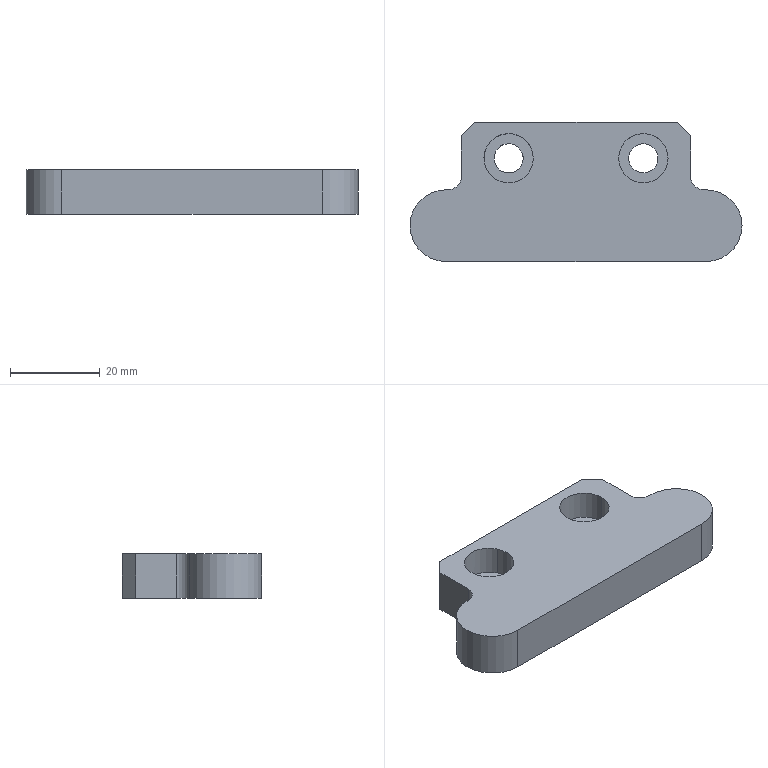Part | STEP file | 1_id1094_x_t | 1 solid | 28 faces | box 73.936 x 31 x 10 mm | volume 16212 mm3 | cylinder 16 | plane 12 | commonest cylinder face diameters 6.5 x4 11 x4 12 x4 6 x2 16 x2